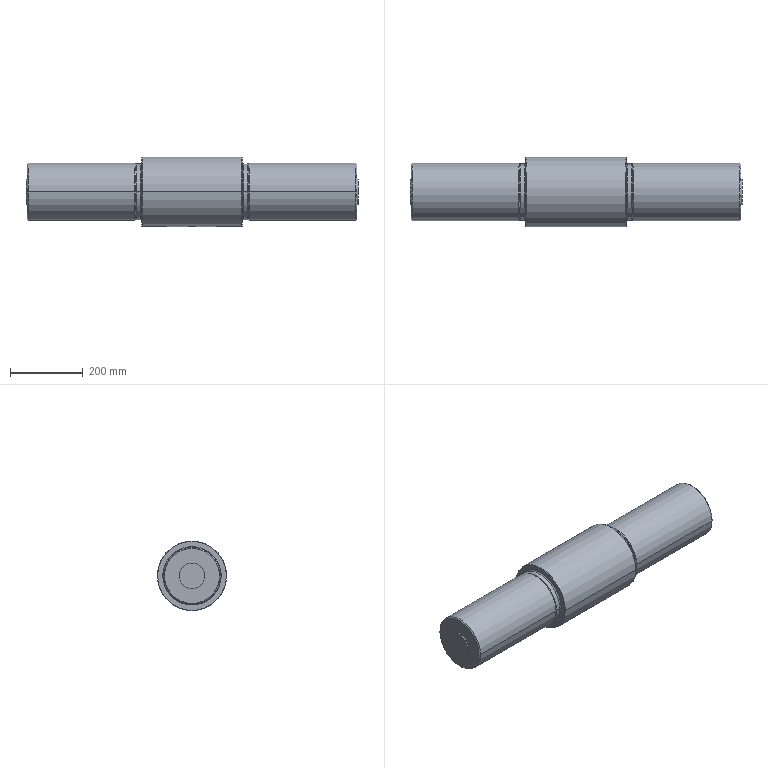Part | SolidWorks | features Chamfer 2, Cut 1, Fillet 1, Revolution 1 | 1 solid | 43 faces | box 909.904 x 190.424 x 190.424 mm | volume 20016200 mm3 | cylinder 16 | cone 12 | torus 8 | plane 7 | commonest cylinder face diameters 69.85 x4 154 x4 157.264 x4 22.631 x2 190.424 x2
STEP:
#1=CARTESIAN_POINT('',(0.,-11.316,-66.51));
#2=VERTEX_POINT('',#1);
#3=CARTESIAN_POINT('',(0.,11.316,-66.51));
#4=VERTEX_POINT('',#3);
#5=CARTESIAN_POINT('',(0.,0.,-66.51));
#6=DIRECTION('',(0.,0.,-1.));
#7=DIRECTION('',(0.,1.,0.));
#8=AXIS2_PLACEMENT_3D('',#5,#6,#7);
#9=CIRCLE('',#8,11.316);
#10=EDGE_CURVE('',#2,#4,#9,.T.);
#11=ORIENTED_EDGE('',*,*,#10,.F.);
#12=CARTESIAN_POINT('',(0.,-11.316,-94.537));
#13=VERTEX_POINT('',#12);
#14=CARTESIAN_POINT('',(0.,-11.316,-66.51));
#15=DIRECTION('',(0.,0.,-1.));
#16=VECTOR('',#15,1000.);
#17=LINE('',#14,#16);
#18=EDGE_CURVE('',#2,#13,#17,.T.);
#19=ORIENTED_EDGE('',*,*,#18,.T.);
#20=CARTESIAN_POINT('',(0.,11.316,-94.537));
#21=VERTEX_POINT('',#20);
#22=CARTESIAN_POINT('',(0.,11.316,-94.537));
#23=CARTESIAN_POINT('',(-0.7484,11.316,-94.537));
#24=CARTESIAN_POINT('',(-1.484,11.242,-94.546));
#25=CARTESIAN_POINT('',(-2.57,11.026,-94.571));
#26=CARTESIAN_POINT('',(-2.928,10.937,-94.582));
#27=CARTESIAN_POINT('',(-3.64,10.721,-94.606));
#28=CARTESIAN_POINT('',(-3.993,10.594,-94.621));
#29=CARTESIAN_POINT('',(-5.021,10.168,-94.668));
#30=CARTESIAN_POINT('',(-5.67,9.82,-94.705));
#31=CARTESIAN_POINT('',(-6.593,9.204,-94.766));
#32=CARTESIAN_POINT('',(-6.892,8.982,-94.788));
#33=CARTESIAN_POINT('',(-7.468,8.509,-94.831));
#34=CARTESIAN_POINT('',(-7.742,8.261,-94.853));
#35=CARTESIAN_POINT('',(-8.524,7.478,-94.919));
#36=CARTESIAN_POINT('',(-8.993,6.909,-94.963));
#37=CARTESIAN_POINT('',(-9.613,5.981,-95.024));
#38=CARTESIAN_POINT('',(-9.805,5.66,-95.044));
#39=CARTESIAN_POINT('',(-10.154,5.007,-95.081));
#40=CARTESIAN_POINT('',(-10.47,4.34,-95.115));
#41=CARTESIAN_POINT('',(-10.719,3.646,-95.143));
#42=CARTESIAN_POINT('',(-10.934,2.937,-95.167));
#43=CARTESIAN_POINT('',(-11.025,2.573,-95.178));
#44=CARTESIAN_POINT('',(-11.244,1.478,-95.203));
#45=CARTESIAN_POINT('',(-11.315,0.7429,-95.212));
#46=CARTESIAN_POINT('',(-11.316,-0.3652,-95.212));
#47=CARTESIAN_POINT('',(-11.298,-0.7357,-95.21));
#48=CARTESIAN_POINT('',(-11.225,-1.479,-95.201));
#49=CARTESIAN_POINT('',(-11.17,-1.848,-95.195));
#50=CARTESIAN_POINT('',(-10.953,-2.937,-95.169));
#51=CARTESIAN_POINT('',(-10.739,-3.643,-95.145));
#52=CARTESIAN_POINT('',(-10.313,-4.671,-95.098));
#53=CARTESIAN_POINT('',(-10.153,-5.01,-95.081));
#54=CARTESIAN_POINT('',(-9.803,-5.665,-95.044));
#55=CARTESIAN_POINT('',(-9.613,-5.982,-95.024));
#56=CARTESIAN_POINT('',(-8.998,-6.901,-94.963));
#57=CARTESIAN_POINT('',(-8.53,-7.472,-94.92));
#58=CARTESIAN_POINT('',(-7.474,-8.529,-94.831));
#59=CARTESIAN_POINT('',(-6.903,-8.996,-94.787));
#60=CARTESIAN_POINT('',(-5.985,-9.611,-94.726));
#61=CARTESIAN_POINT('',(-5.668,-9.801,-94.706));
#62=CARTESIAN_POINT('',(-5.013,-10.151,-94.669));
#63=CARTESIAN_POINT('',(-4.674,-10.312,-94.652));
#64=CARTESIAN_POINT('',(-3.646,-10.738,-94.605));
#65=CARTESIAN_POINT('',(-2.941,-10.952,-94.58));
#66=CARTESIAN_POINT('',(-1.852,-11.169,-94.555));
#67=CARTESIAN_POINT('',(-1.483,-11.224,-94.548));
#68=CARTESIAN_POINT('',(-0.7399,-11.298,-94.539));
#69=CARTESIAN_POINT('',(-0.3694,-11.316,-94.537));
#70=CARTESIAN_POINT('',(0.,-11.316,-94.537));
#71=B_SPLINE_CURVE_WITH_KNOTS('',3,(#22,#23,#24,#25,#26,#27,#28,#29,#30,#31,#32,#33,#34,#35,#36,#37,#38,#39,#40,#41,#42,#43,#44,#45,#46,#47,#48,#49,#50,#51,#52,#53,#54,#55,#56,#57,#58,#59,#60,#61,#62,#63,#64,#65,#66,#67,#68,#69,#70),.UNSPECIFIED.,.F.,.F.,(4,2,2,2,2,2,2,2,2,1,2,2,2,2,2,2,2,2,2,2,2,2,2,2,4),(0.,0.002213,0.00332,0.004426,0.006639,0.007746,0.008852,0.01107,0.01217,0.01328,0.01439,0.01549,0.0177,0.01881,0.01992,0.02213,0.02324,0.02434,0.02656,0.02877,0.02988,0.03098,0.0332,0.0343,0.03541),.UNSPECIFIED.);
#72=EDGE_CURVE('',#21,#13,#71,.T.);
#73=ORIENTED_EDGE('',*,*,#72,.F.);
#74=CARTESIAN_POINT('',(0.,11.316,-66.51));
#75=DIRECTION('',(0.,0.,-1.));
#76=VECTOR('',#75,1000.);
#77=LINE('',#74,#76);
#78=EDGE_CURVE('',#4,#21,#77,.T.);
#79=ORIENTED_EDGE('',*,*,#78,.F.);
#80=EDGE_LOOP('',(#11,#19,#73,#79));
#81=FACE_OUTER_BOUND('',#80,.T.);
#82=CARTESIAN_POINT('',(0.,0.,-66.51));
#83=DIRECTION('',(0.,0.,-1.));
#84=DIRECTION('',(0.,1.,0.));
#85=AXIS2_PLACEMENT_3D('',#82,#83,#84);
#86=CYLINDRICAL_SURFACE('',#85,11.316);
#87=ADVANCED_FACE('',(#81),#86,.F.);
#88=CARTESIAN_POINT('',(-137.325,-80.175,0.));
#89=VERTEX_POINT('',#88);
#90=CARTESIAN_POINT('',(-137.325,80.175,0.));
#91=VERTEX_POINT('',#90);
#92=CARTESIAN_POINT('',(-137.325,0.,0.));
#93=DIRECTION('',(1.,0.,0.));
#94=DIRECTION('',(0.,1.,0.));
#95=AXIS2_PLACEMENT_3D('',#92,#93,#94);
#96=CIRCLE('',#95,80.175);
#97=EDGE_CURVE('',#89,#91,#96,.T.);
#98=ORIENTED_EDGE('',*,*,#97,.F.);
#99=CARTESIAN_POINT('',(-140.5,-77.,0.));
#100=VERTEX_POINT('',#99);
#101=CARTESIAN_POINT('',(-140.5,-80.175,0.));
#102=DIRECTION('',(0.,0.,1.));
#103=DIRECTION('',(0.,-1.,0.));
#104=AXIS2_PLACEMENT_3D('',#101,#102,#103);
#105=CIRCLE('',#104,3.175);
#106=EDGE_CURVE('',#89,#100,#105,.T.);
#107=ORIENTED_EDGE('',*,*,#106,.T.);
#108=CARTESIAN_POINT('',(-140.5,77.,0.));
#109=VERTEX_POINT('',#108);
#110=CARTESIAN_POINT('',(-140.5,0.,0.));
#111=DIRECTION('',(-1.,0.,0.));
#112=DIRECTION('',(0.,1.,0.));
#113=AXIS2_PLACEMENT_3D('',#110,#111,#112);
#114=CIRCLE('',#113,77.);
#115=EDGE_CURVE('',#109,#100,#114,.T.);
#116=ORIENTED_EDGE('',*,*,#115,.F.);
#117=CARTESIAN_POINT('',(-140.5,80.175,0.));
#118=DIRECTION('',(0.,0.,-1.));
#119=DIRECTION('',(-1.,0.,0.));
#120=AXIS2_PLACEMENT_3D('',#117,#118,#119);
#121=CIRCLE('',#120,3.175);
#122=EDGE_CURVE('',#91,#109,#121,.T.);
#123=ORIENTED_EDGE('',*,*,#122,.F.);
#124=EDGE_LOOP('',(#98,#107,#116,#123));
#125=FACE_OUTER_BOUND('',#124,.T.);
#126=CARTESIAN_POINT('',(-140.5,0.,0.));
#127=DIRECTION('',(1.,0.,0.));
#128=DIRECTION('',(0.,1.,0.));
#129=AXIS2_PLACEMENT_3D('',#126,#127,#128);
#130=TOROIDAL_SURFACE('',#129,80.175,3.175);
#131=ADVANCED_FACE('',(#125),#130,.F.);
#132=CARTESIAN_POINT('',(-154.285,77.425,0.));
#133=VERTEX_POINT('',#132);
#134=CARTESIAN_POINT('',(-154.285,-77.425,0.));
#135=VERTEX_POINT('',#134);
#136=CARTESIAN_POINT('',(-154.285,0.,0.));
#137=DIRECTION('',(-1.,0.,0.));
#138=DIRECTION('',(0.,-1.,0.));
#139=AXIS2_PLACEMENT_3D('',#136,#137,#138);
#140=CIRCLE('',#139,77.425);
#141=EDGE_CURVE('',#133,#135,#140,.T.);
#142=ORIENTED_EDGE('',*,*,#141,.F.);
#143=CARTESIAN_POINT('',(-152.698,77.,0.));
#144=VERTEX_POINT('',#143);
#145=CARTESIAN_POINT('',(-152.698,80.175,0.));
#146=DIRECTION('',(0.,0.,1.));
#147=DIRECTION('',(0.,-1.,0.));
#148=AXIS2_PLACEMENT_3D('',#145,#146,#147);
#149=CIRCLE('',#148,3.175);
#150=EDGE_CURVE('',#133,#144,#149,.T.);
#151=ORIENTED_EDGE('',*,*,#150,.T.);
#152=CARTESIAN_POINT('',(-152.698,-77.,0.));
#153=VERTEX_POINT('',#152);
#154=CARTESIAN_POINT('',(-152.698,0.,0.));
#155=DIRECTION('',(1.,0.,0.));
#156=DIRECTION('',(0.,-1.,0.));
#157=AXIS2_PLACEMENT_3D('',#154,#155,#156);
#158=CIRCLE('',#157,77.);
#159=EDGE_CURVE('',#153,#144,#158,.T.);
#160=ORIENTED_EDGE('',*,*,#159,.F.);
#161=CARTESIAN_POINT('',(-152.698,-80.175,0.));
#162=DIRECTION('',(0.,0.,-1.));
#163=DIRECTION('',(-1.,0.,0.));
#164=AXIS2_PLACEMENT_3D('',#161,#162,#163);
#165=CIRCLE('',#164,3.175);
#166=EDGE_CURVE('',#135,#153,#165,.T.);
#167=ORIENTED_EDGE('',*,*,#166,.F.);
#168=EDGE_LOOP('',(#142,#151,#160,#167));
#169=FACE_OUTER_BOUND('',#168,.T.);
#170=CARTESIAN_POINT('',(-152.698,0.,0.));
#171=DIRECTION('',(-1.,0.,0.));
#172=DIRECTION('',(0.,-1.,0.));
#173=AXIS2_PLACEMENT_3D('',#170,#171,#172);
#174=TOROIDAL_SURFACE('',#173,80.175,3.175);
#175=ADVANCED_FACE('',(#169),#174,.F.);
#176=CARTESIAN_POINT('',(137.325,80.175,0.));
#177=VERTEX_POINT('',#176);
#178=CARTESIAN_POINT('',(137.325,-80.175,0.));
#179=VERTEX_POINT('',#178);
#180=CARTESIAN_POINT('',(137.325,0.,0.));
#181=DIRECTION('',(-1.,0.,0.));
#182=DIRECTION('',(0.,-1.,0.));
#183=AXIS2_PLACEMENT_3D('',#180,#181,#182);
#184=CIRCLE('',#183,80.175);
#185=EDGE_CURVE('',#177,#179,#184,.T.);
#186=ORIENTED_EDGE('',*,*,#185,.F.);
#187=CARTESIAN_POINT('',(140.5,77.,0.));
#188=VERTEX_POINT('',#187);
#189=CARTESIAN_POINT('',(140.5,80.175,0.));
#190=DIRECTION('',(0.,0.,1.));
#191=DIRECTION('',(0.,-1.,0.));
#192=AXIS2_PLACEMENT_3D('',#189,#190,#191);
#193=CIRCLE('',#192,3.175);
#194=EDGE_CURVE('',#177,#188,#193,.T.);
#195=ORIENTED_EDGE('',*,*,#194,.T.);
#196=CARTESIAN_POINT('',(140.5,-77.,0.));
#197=VERTEX_POINT('',#196);
#198=CARTESIAN_POINT('',(140.5,0.,0.));
#199=DIRECTION('',(1.,0.,0.));
#200=DIRECTION('',(0.,-1.,0.));
#201=AXIS2_PLACEMENT_3D('',#198,#199,#200);
#202=CIRCLE('',#201,77.);
#203=EDGE_CURVE('',#197,#188,#202,.T.);
#204=ORIENTED_EDGE('',*,*,#203,.F.);
#205=CARTESIAN_POINT('',(140.5,-80.175,0.));
#206=DIRECTION('',(0.,0.,-1.));
#207=DIRECTION('',(-1.,0.,0.));
#208=AXIS2_PLACEMENT_3D('',#205,#206,#207);
#209=CIRCLE('',#208,3.175);
#210=EDGE_CURVE('',#179,#197,#209,.T.);
#211=ORIENTED_EDGE('',*,*,#210,.F.);
#212=EDGE_LOOP('',(#186,#195,#204,#211));
#213=FACE_OUTER_BOUND('',#212,.T.);
#214=CARTESIAN_POINT('',(140.5,0.,0.));
#215=DIRECTION('',(-1.,0.,0.));
#216=DIRECTION('',(0.,-1.,0.));
#217=AXIS2_PLACEMENT_3D('',#214,#215,#216);
#218=TOROIDAL_SURFACE('',#217,80.175,3.175);
#219=ADVANCED_FACE('',(#213),#218,.F.);
#220=CARTESIAN_POINT('',(152.698,77.,0.));
#221=VERTEX_POINT('',#220);
#222=CARTESIAN_POINT('',(152.698,-77.,0.));
#223=VERTEX_POINT('',#222);
#224=CARTESIAN_POINT('',(152.698,0.,0.));
#225=DIRECTION('',(-1.,0.,0.));
#226=DIRECTION('',(0.,-1.,0.));
#227=AXIS2_PLACEMENT_3D('',#224,#225,#226);
#228=CIRCLE('',#227,77.);
#229=EDGE_CURVE('',#221,#223,#228,.T.);
#230=ORIENTED_EDGE('',*,*,#229,.F.);
#231=CARTESIAN_POINT('',(154.285,77.425,0.));
#232=VERTEX_POINT('',#231);
#233=CARTESIAN_POINT('',(152.698,80.175,0.));
#234=DIRECTION('',(0.,0.,1.));
#235=DIRECTION('',(0.,-1.,0.));
#236=AXIS2_PLACEMENT_3D('',#233,#234,#235);
#237=CIRCLE('',#236,3.175);
#238=EDGE_CURVE('',#221,#232,#237,.T.);
#239=ORIENTED_EDGE('',*,*,#238,.T.);
#240=CARTESIAN_POINT('',(154.285,-77.425,0.));
#241=VERTEX_POINT('',#240);
#242=CARTESIAN_POINT('',(154.285,0.,0.));
#243=DIRECTION('',(1.,0.,0.));
#244=DIRECTION('',(0.,1.,0.));
#245=AXIS2_PLACEMENT_3D('',#242,#243,#244);
#246=CIRCLE('',#245,77.425);
#247=EDGE_CURVE('',#241,#232,#246,.T.);
#248=ORIENTED_EDGE('',*,*,#247,.F.);
#249=CARTESIAN_POINT('',(152.698,-80.175,0.));
#250=DIRECTION('',(0.,0.,-1.));
#251=DIRECTION('',(-1.,0.,0.));
#252=AXIS2_PLACEMENT_3D('',#249,#250,#251);
#253=CIRCLE('',#252,3.175);
#254=EDGE_CURVE('',#223,#241,#253,.T.);
#255=ORIENTED_EDGE('',*,*,#254,.F.);
#256=EDGE_LOOP('',(#230,#239,#248,#255));
#257=FACE_OUTER_BOUND('',#256,.T.);
#258=CARTESIAN_POINT('',(152.698,0.,0.));
#259=DIRECTION('',(-1.,0.,0.));
#260=DIRECTION('',(0.,-1.,0.));
#261=AXIS2_PLACEMENT_3D('',#258,#259,#260);
#262=TOROIDAL_SURFACE('',#261,80.175,3.175);
#263=ADVANCED_FACE('',(#257),#262,.F.);
#264=CARTESIAN_POINT('',(-137.325,-94.45,0.));
#265=VERTEX_POINT('',#264);
#266=CARTESIAN_POINT('',(-137.325,94.45,0.));
#267=VERTEX_POINT('',#266);
#268=CARTESIAN_POINT('',(-137.325,0.,0.));
#269=DIRECTION('',(-1.,0.,0.));
#270=DIRECTION('',(0.,1.,0.));
#271=AXIS2_PLACEMENT_3D('',#268,#269,#270);
#272=CIRCLE('',#271,94.45);
#273=EDGE_CURVE('',#265,#267,#272,.T.);
#274=ORIENTED_EDGE('',*,*,#273,.F.);
#275=CARTESIAN_POINT('',(-136.563,-95.212,0.));
#276=VERTEX_POINT('',#275);
#277=CARTESIAN_POINT('',(-137.325,-94.45,0.));
#278=DIRECTION('',(0.7071,-0.7071,0.));
#279=VECTOR('',#278,1000.);
#280=LINE('',#277,#279);
#281=EDGE_CURVE('',#265,#276,#280,.T.);
#282=ORIENTED_EDGE('',*,*,#281,.T.);
#283=CARTESIAN_POINT('',(-136.563,95.212,0.));
#284=VERTEX_POINT('',#283);
#285=CARTESIAN_POINT('',(-136.563,0.,0.));
#286=DIRECTION('',(1.,0.,0.));
#287=DIRECTION('',(0.,1.,0.));
#288=AXIS2_PLACEMENT_3D('',#285,#286,#287);
#289=CIRCLE('',#288,95.212);
#290=EDGE_CURVE('',#284,#276,#289,.T.);
#291=ORIENTED_EDGE('',*,*,#290,.F.);
#292=CARTESIAN_POINT('',(-137.325,94.45,0.));
#293=DIRECTION('',(0.7071,0.7071,0.));
#294=VECTOR('',#293,1000.);
#295=LINE('',#292,#294);
#296=EDGE_CURVE('',#267,#284,#295,.T.);
#297=ORIENTED_EDGE('',*,*,#296,.F.);
#298=EDGE_LOOP('',(#274,#282,#291,#297));
#299=FACE_OUTER_BOUND('',#298,.T.);
#300=CARTESIAN_POINT('',(-137.325,0.,0.));
#301=DIRECTION('',(1.,0.,0.));
#302=DIRECTION('',(0.,1.,0.));
#303=AXIS2_PLACEMENT_3D('',#300,#301,#302);
#304=CONICAL_SURFACE('',#303,94.45,0.7854);
#305=ADVANCED_FACE('',(#299),#304,.T.);
#306=CARTESIAN_POINT('',(137.325,94.45,0.));
#307=VERTEX_POINT('',#306);
#308=CARTESIAN_POINT('',(137.325,-94.45,0.));
#309=VERTEX_POINT('',#308);
#310=CARTESIAN_POINT('',(137.325,0.,0.));
#311=DIRECTION('',(1.,0.,0.));
#312=DIRECTION('',(0.,-1.,0.));
#313=AXIS2_PLACEMENT_3D('',#310,#311,#312);
#314=CIRCLE('',#313,94.45);
#315=EDGE_CURVE('',#307,#309,#314,.T.);
#316=ORIENTED_EDGE('',*,*,#315,.F.);
#317=CARTESIAN_POINT('',(136.563,95.212,0.));
#318=VERTEX_POINT('',#317);
#319=CARTESIAN_POINT('',(136.563,95.212,0.));
#320=DIRECTION('',(-0.7071,0.7071,0.));
#321=VECTOR('',#320,1000.);
#322=LINE('',#319,#321);
#323=EDGE_CURVE('',#307,#318,#322,.T.);
#324=ORIENTED_EDGE('',*,*,#323,.T.);
#325=CARTESIAN_POINT('',(136.563,-95.212,0.));
#326=VERTEX_POINT('',#325);
#327=CARTESIAN_POINT('',(136.563,0.,0.));
#328=DIRECTION('',(-1.,0.,0.));
#329=DIRECTION('',(0.,-1.,0.));
#330=AXIS2_PLACEMENT_3D('',#327,#328,#329);
#331=CIRCLE('',#330,95.212);
#332=EDGE_CURVE('',#326,#318,#331,.T.);
#333=ORIENTED_EDGE('',*,*,#332,.F.);
#334=CARTESIAN_POINT('',(136.563,-95.212,0.));
#335=DIRECTION('',(-0.7071,-0.7071,0.));
#336=VECTOR('',#335,1000.);
#337=LINE('',#334,#336);
#338=EDGE_CURVE('',#309,#326,#337,.T.);
#339=ORIENTED_EDGE('',*,*,#338,.F.);
#340=EDGE_LOOP('',(#316,#324,#333,#339));
#341=FACE_OUTER_BOUND('',#340,.T.);
#342=CARTESIAN_POINT('',(136.563,0.,0.));
#343=DIRECTION('',(-1.,0.,0.));
#344=DIRECTION('',(0.,-1.,0.));
#345=AXIS2_PLACEMENT_3D('',#342,#343,#344);
#346=CONICAL_SURFACE('',#345,95.212,0.7854);
#347=ADVANCED_FACE('',(#341),#346,.T.);
#348=CARTESIAN_POINT('',(-451.65,-75.632,0.));
#349=VERTEX_POINT('',#348);
#350=CARTESIAN_POINT('',(-451.65,75.632,0.));
#351=VERTEX_POINT('',#350);
#352=CARTESIAN_POINT('',(-451.65,0.,0.));
#353=DIRECTION('',(-1.,0.,0.));
#354=DIRECTION('',(0.,1.,0.));
#355=AXIS2_PLACEMENT_3D('',#352,#353,#354);
#356=CIRCLE('',#355,75.632);
#357=EDGE_CURVE('',#349,#351,#356,.T.);
#358=ORIENTED_EDGE('',*,*,#357,.F.);
#359=CARTESIAN_POINT('',(-448.65,-78.632,0.));
#360=VERTEX_POINT('',#359);
#361=CARTESIAN_POINT('',(-451.65,-75.632,0.));
#362=DIRECTION('',(0.7071,-0.7071,0.));
#363=VECTOR('',#362,1000.);
#364=LINE('',#361,#363);
#365=EDGE_CURVE('',#349,#360,#364,.T.);
#366=ORIENTED_EDGE('',*,*,#365,.T.);
#367=CARTESIAN_POINT('',(-448.65,78.632,0.));
#368=VERTEX_POINT('',#367);
#369=CARTESIAN_POINT('',(-448.65,0.,0.));
#370=DIRECTION('',(1.,0.,0.));
#371=DIRECTION('',(0.,1.,0.));
#372=AXIS2_PLACEMENT_3D('',#369,#370,#371);
#373=CIRCLE('',#372,78.632);
#374=EDGE_CURVE('',#368,#360,#373,.T.);
#375=ORIENTED_EDGE('',*,*,#374,.F.);
#376=CARTESIAN_POINT('',(-451.65,75.632,0.));
#377=DIRECTION('',(0.7071,0.7071,0.));
#378=VECTOR('',#377,1000.);
#379=LINE('',#376,#378);
#380=EDGE_CURVE('',#351,#368,#379,.T.);
#381=ORIENTED_EDGE('',*,*,#380,.F.);
#382=EDGE_LOOP('',(#358,#366,#375,#381));
#383=FACE_OUTER_BOUND('',#382,.T.);
#384=CARTESIAN_POINT('',(-451.65,0.,0.));
#385=DIRECTION('',(1.,0.,0.));
#386=DIRECTION('',(0.,1.,0.));
#387=AXIS2_PLACEMENT_3D('',#384,#385,#386);
#388=CONICAL_SURFACE('',#387,75.632,0.7854);
#389=ADVANCED_FACE('',(#383),#388,.T.);
#390=CARTESIAN_POINT('',(451.65,75.632,0.));
#391=VERTEX_POINT('',#390);
#392=CARTESIAN_POINT('',(451.65,-75.632,0.));
#393=VERTEX_POINT('',#392);
#394=CARTESIAN_POINT('',(451.65,0.,0.));
#395=DIRECTION('',(1.,0.,0.));
#396=DIRECTION('',(0.,-1.,0.));
#397=AXIS2_PLACEMENT_3D('',#394,#395,#396);
#398=CIRCLE('',#397,75.632);
#399=EDGE_CURVE('',#391,#393,#398,.T.);
#400=ORIENTED_EDGE('',*,*,#399,.F.);
#401=CARTESIAN_POINT('',(448.65,78.632,0.));
#402=VERTEX_POINT('',#401);
#403=CARTESIAN_POINT('',(448.65,78.632,0.));
#404=DIRECTION('',(-0.7071,0.7071,0.));
#405=VECTOR('',#404,1000.);
#406=LINE('',#403,#405);
#407=EDGE_CURVE('',#391,#402,#406,.T.);
#408=ORIENTED_EDGE('',*,*,#407,.T.);
#409=CARTESIAN_POINT('',(448.65,-78.632,0.));
#410=VERTEX_POINT('',#409);
#411=CARTESIAN_POINT('',(448.65,0.,0.));
#412=DIRECTION('',(-1.,0.,0.));
#413=DIRECTION('',(0.,-1.,0.));
#414=AXIS2_PLACEMENT_3D('',#411,#412,#413);
#415=CIRCLE('',#414,78.632);
#416=EDGE_CURVE('',#410,#402,#415,.T.);
#417=ORIENTED_EDGE('',*,*,#416,.F.);
#418=CARTESIAN_POINT('',(448.65,-78.632,0.));
#419=DIRECTION('',(-0.7071,-0.7071,0.));
#420=VECTOR('',#419,1000.);
#421=LINE('',#418,#420);
#422=EDGE_CURVE('',#393,#410,#421,.T.);
#423=ORIENTED_EDGE('',*,*,#422,.F.);
#424=EDGE_LOOP('',(#400,#408,#417,#423));
#425=FACE_OUTER_BOUND('',#424,.T.);
#426=CARTESIAN_POINT('',(448.65,0.,0.));
#427=DIRECTION('',(-1.,0.,0.));
#428=DIRECTION('',(0.,-1.,0.));
#429=AXIS2_PLACEMENT_3D('',#426,#427,#428);
#430=CONICAL_SURFACE('',#429,78.632,0.7854);
#431=ADVANCED_FACE('',(#425),#430,.T.);
#432=CARTESIAN_POINT('',(154.285,0.,0.));
#433=DIRECTION('',(1.,0.,0.));
#434=DIRECTION('',(0.,1.,0.));
#435=AXIS2_PLACEMENT_3D('',#432,#433,#434);
#436=CIRCLE('',#435,77.425);
#437=EDGE_CURVE('',#232,#241,#436,.T.);
#438=ORIENTED_EDGE('',*,*,#437,.T.);
#439=CARTESIAN_POINT('',(156.375,-78.632,0.));
#440=VERTEX_POINT('',#439);
#441=CARTESIAN_POINT('',(156.375,-78.632,0.));
#442=DIRECTION('',(0.866,-0.5,0.));
#443=VECTOR('',#442,1000.);
#444=LINE('',#441,#443);
#445=EDGE_CURVE('',#241,#440,#444,.T.);
#446=ORIENTED_EDGE('',*,*,#445,.T.);
#447=CARTESIAN_POINT('',(156.375,78.632,0.));
#448=VERTEX_POINT('',#447);
#449=CARTESIAN_POINT('',(156.375,0.,0.));
#450=DIRECTION('',(-1.,0.,0.));
#451=DIRECTION('',(0.,-1.,0.));
#452=AXIS2_PLACEMENT_3D('',#449,#450,#451);
#453=CIRCLE('',#452,78.632);
#454=EDGE_CURVE('',#440,#448,#453,.T.);
#455=ORIENTED_EDGE('',*,*,#454,.T.);
#456=CARTESIAN_POINT('',(156.375,78.632,0.));
#457=DIRECTION('',(0.866,0.5,0.));
#458=VECTOR('',#457,1000.);
#459=LINE('',#456,#458);
#460=EDGE_CURVE('',#232,#448,#459,.T.);
#461=ORIENTED_EDGE('',*,*,#460,.F.);
#462=EDGE_LOOP('',(#438,#446,#455,#461));
#463=FACE_OUTER_BOUND('',#462,.T.);
#464=CARTESIAN_POINT('',(156.375,0.,0.));
#465=DIRECTION('',(1.,0.,0.));
#466=DIRECTION('',(0.,1.,0.));
#467=AXIS2_PLACEMENT_3D('',#464,#465,#466);
#468=CONICAL_SURFACE('',#467,78.632,0.5236);
#469=ADVANCED_FACE('',(#463),#468,.T.);
#470=CARTESIAN_POINT('',(152.698,0.,0.));
#471=DIRECTION('',(-1.,0.,0.));
#472=DIRECTION('',(0.,-1.,0.));
#473=AXIS2_PLACEMENT_3D('',#470,#471,#472);
#474=CIRCLE('',#473,77.);
#475=EDGE_CURVE('',#223,#221,#474,.T.);
#476=ORIENTED_EDGE('',*,*,#475,.T.);
#477=CARTESIAN_POINT('',(-454.952,77.,0.));
#478=DIRECTION('',(-1.,0.,0.));
#479=VECTOR('',#478,1000.);
#480=LINE('',#477,#479);
#481=EDGE_CURVE('',#221,#188,#480,.T.);
#482=ORIENTED_EDGE('',*,*,#481,.T.);
#483=CARTESIAN_POINT('',(140.5,0.,0.));
#484=DIRECTION('',(1.,0.,0.));
#485=DIRECTION('',(0.,-1.,0.));
#486=AXIS2_PLACEMENT_3D('',#483,#484,#485);
#487=CIRCLE('',#486,77.);
#488=EDGE_CURVE('',#188,#197,#487,.T.);
#489=ORIENTED_EDGE('',*,*,#488,.T.);
#490=CARTESIAN_POINT('',(-454.952,-77.,0.));
#491=DIRECTION('',(-1.,0.,0.));
#492=VECTOR('',#491,1000.);
#493=LINE('',#490,#492);
#494=EDGE_CURVE('',#223,#197,#493,.T.);
#495=ORIENTED_EDGE('',*,*,#494,.F.);
#496=EDGE_LOOP('',(#476,#482,#489,#495));
#497=FACE_OUTER_BOUND('',#496,.T.);
#498=CARTESIAN_POINT('',(-454.952,0.,0.));
#499=DIRECTION('',(-1.,0.,0.));
#500=DIRECTION('',(0.,-1.,0.));
#501=AXIS2_PLACEMENT_3D('',#498,#499,#500);
#502=CYLINDRICAL_SURFACE('',#501,77.);
#503=ADVANCED_FACE('',(#497),#502,.T.);
#504=ORIENTED_EDGE('',*,*,#332,.T.);
#505=CARTESIAN_POINT('',(-454.952,95.212,0.));
#506=DIRECTION('',(-1.,0.,0.));
#507=VECTOR('',#506,1000.);
#508=LINE('',#505,#507);
#509=EDGE_CURVE('',#318,#284,#508,.T.);
#510=ORIENTED_EDGE('',*,*,#509,.T.);
#511=ORIENTED_EDGE('',*,*,#290,.T.);
#512=CARTESIAN_POINT('',(-454.952,-95.212,0.));
#513=DIRECTION('',(-1.,0.,0.));
#514=VECTOR('',#513,1000.);
#515=LINE('',#512,#514);
#516=EDGE_CURVE('',#326,#276,#515,.T.);
#517=ORIENTED_EDGE('',*,*,#516,.F.);
#518=EDGE_LOOP('',(#504,#510,#511,#517));
#519=FACE_OUTER_BOUND('',#518,.T.);
#520=CARTESIAN_POINT('',(-454.952,0.,0.));
#521=DIRECTION('',(-1.,0.,0.));
#522=DIRECTION('',(0.,-1.,0.));
#523=AXIS2_PLACEMENT_3D('',#520,#521,#522);
#524=CYLINDRICAL_SURFACE('',#523,95.212);
#525=ADVANCED_FACE('',(#519),#524,.T.);
#526=CARTESIAN_POINT('',(-140.5,0.,0.));
#527=DIRECTION('',(-1.,0.,0.));
#528=DIRECTION('',(0.,1.,0.));
#529=AXIS2_PLACEMENT_3D('',#526,#527,#528);
#530=CIRCLE('',#529,77.);
#531=EDGE_CURVE('',#100,#109,#530,.T.);
#532=ORIENTED_EDGE('',*,*,#531,.T.);
#533=CARTESIAN_POINT('',(-454.952,77.,0.));
#534=DIRECTION('',(-1.,0.,0.));
#535=VECTOR('',#534,1000.);
#536=LINE('',#533,#535);
#537=EDGE_CURVE('',#109,#144,#536,.T.);
#538=ORIENTED_EDGE('',*,*,#537,.T.);
#539=CARTESIAN_POINT('',(-152.698,0.,0.));
#540=DIRECTION('',(1.,0.,0.));
#541=DIRECTION('',(0.,-1.,0.));
#542=AXIS2_PLACEMENT_3D('',#539,#540,#541);
#543=CIRCLE('',#542,77.);
#544=EDGE_CURVE('',#144,#153,#543,.T.);
#545=ORIENTED_EDGE('',*,*,#544,.T.);
#546=CARTESIAN_POINT('',(-454.952,-77.,0.));
#547=DIRECTION('',(-1.,0.,0.));
#548=VECTOR('',#547,1000.);
#549=LINE('',#546,#548);
#550=EDGE_CURVE('',#100,#153,#549,.T.);
#551=ORIENTED_EDGE('',*,*,#550,.F.);
#552=EDGE_LOOP('',(#532,#538,#545,#551));
#553=FACE_OUTER_BOUND('',#552,.T.);
#554=CARTESIAN_POINT('',(-454.952,0.,0.));
#555=DIRECTION('',(-1.,0.,0.));
#556=DIRECTION('',(0.,-1.,0.));
#557=AXIS2_PLACEMENT_3D('',#554,#555,#556);
#558=CYLINDRICAL_SURFACE('',#557,77.);
#559=ADVANCED_FACE('',(#553),#558,.T.);
#560=CARTESIAN_POINT('',(-154.285,0.,0.));
#561=DIRECTION('',(-1.,0.,0.));
#562=DIRECTION('',(0.,-1.,0.));
#563=AXIS2_PLACEMENT_3D('',#560,#561,#562);
#564=CIRCLE('',#563,77.425);
#565=EDGE_CURVE('',#135,#133,#564,.T.);
#566=ORIENTED_EDGE('',*,*,#565,.T.);
#567=CARTESIAN_POINT('',(-156.375,78.632,0.));
#568=VERTEX_POINT('',#567);
#569=CARTESIAN_POINT('',(-153.548,77.,0.));
#570=DIRECTION('',(-0.866,0.5,0.));
#571=VECTOR('',#570,1000.);
#572=LINE('',#569,#571);
#573=EDGE_CURVE('',#133,#568,#572,.T.);
#574=ORIENTED_EDGE('',*,*,#573,.T.);
#575=CARTESIAN_POINT('',(-156.375,-78.632,0.));
#576=VERTEX_POINT('',#575);
#577=CARTESIAN_POINT('',(-156.375,0.,0.));
#578=DIRECTION('',(-1.,0.,0.));
#579=DIRECTION('',(0.,-1.,0.));
#580=AXIS2_PLACEMENT_3D('',#577,#578,#579);
#581=CIRCLE('',#580,78.632);
#582=EDGE_CURVE('',#576,#568,#581,.T.);
#583=ORIENTED_EDGE('',*,*,#582,.F.);
#584=CARTESIAN_POINT('',(-153.548,-77.,0.));
#585=DIRECTION('',(-0.866,-0.5,0.));
#586=VECTOR('',#585,1000.);
#587=LINE('',#584,#586);
#588=EDGE_CURVE('',#135,#576,#587,.T.);
#589=ORIENTED_EDGE('',*,*,#588,.F.);
#590=EDGE_LOOP('',(#566,#574,#583,#589));
#591=FACE_OUTER_BOUND('',#590,.T.);
#592=CARTESIAN_POINT('',(-153.548,0.,0.));
#593=DIRECTION('',(-1.,0.,0.));
#594=DIRECTION('',(0.,-1.,0.));
#595=AXIS2_PLACEMENT_3D('',#592,#593,#594);
#596=CONICAL_SURFACE('',#595,77.,0.5236);
#597=ADVANCED_FACE('',(#591),#596,.T.);
#598=ORIENTED_EDGE('',*,*,#582,.T.);
#599=CARTESIAN_POINT('',(-454.952,78.632,0.));
#600=DIRECTION('',(-1.,0.,0.));
#601=VECTOR('',#600,1000.);
#602=LINE('',#599,#601);
#603=EDGE_CURVE('',#568,#368,#602,.T.);
#604=ORIENTED_EDGE('',*,*,#603,.T.);
#605=ORIENTED_EDGE('',*,*,#374,.T.);
#606=CARTESIAN_POINT('',(-454.952,-78.632,0.));
#607=DIRECTION('',(-1.,0.,0.));
#608=VECTOR('',#607,1000.);
#609=LINE('',#606,#608);
#610=EDGE_CURVE('',#576,#360,#609,.T.);
#611=ORIENTED_EDGE('',*,*,#610,.F.);
#612=EDGE_LOOP('',(#598,#604,#605,#611));
#613=FACE_OUTER_BOUND('',#612,.T.);
#614=CARTESIAN_POINT('',(-454.952,0.,0.));
#615=DIRECTION('',(-1.,0.,0.));
#616=DIRECTION('',(0.,-1.,0.));
#617=AXIS2_PLACEMENT_3D('',#614,#615,#616);
#618=CYLINDRICAL_SURFACE('',#617,78.632);
#619=ADVANCED_FACE('',(#613),#618,.T.);
#620=CARTESIAN_POINT('',(-451.65,-34.925,0.));
#621=VERTEX_POINT('',#620);
#622=CARTESIAN_POINT('',(-451.65,34.925,0.));
#623=VERTEX_POINT('',#622);
#624=CARTESIAN_POINT('',(-451.65,0.,0.));
#625=DIRECTION('',(-1.,0.,0.));
#626=DIRECTION('',(0.,-1.,0.));
#627=AXIS2_PLACEMENT_3D('',#624,#625,#626);
#628=CIRCLE('',#627,34.925);
#629=EDGE_CURVE('',#621,#623,#628,.T.);
#630=ORIENTED_EDGE('',*,*,#629,.T.);
#631=CARTESIAN_POINT('',(-454.952,34.925,0.));
#632=VERTEX_POINT('',#631);
#633=CARTESIAN_POINT('',(-454.952,34.925,0.));
#634=DIRECTION('',(-1.,0.,0.));
#635=VECTOR('',#634,1000.);
#636=LINE('',#633,#635);
#637=EDGE_CURVE('',#623,#632,#636,.T.);
#638=ORIENTED_EDGE('',*,*,#637,.T.);
#639=CARTESIAN_POINT('',(-454.952,-34.925,0.));
#640=VERTEX_POINT('',#639);
#641=CARTESIAN_POINT('',(-454.952,0.,0.));
#642=DIRECTION('',(-1.,0.,0.));
#643=DIRECTION('',(0.,-1.,0.));
#644=AXIS2_PLACEMENT_3D('',#641,#642,#643);
#645=CIRCLE('',#644,34.925);
#646=EDGE_CURVE('',#640,#632,#645,.T.);
#647=ORIENTED_EDGE('',*,*,#646,.F.);
#648=CARTESIAN_POINT('',(-454.952,-34.925,0.));
#649=DIRECTION('',(-1.,0.,0.));
#650=VECTOR('',#649,1000.);
#651=LINE('',#648,#650);
#652=EDGE_CURVE('',#621,#640,#651,.T.);
#653=ORIENTED_EDGE('',*,*,#652,.F.);
#654=EDGE_LOOP('',(#630,#638,#647,#653));
#655=FACE_OUTER_BOUND('',#654,.T.);
#656=CARTESIAN_POINT('',(-454.952,0.,0.));
#657=DIRECTION('',(-1.,0.,0.));
#658=DIRECTION('',(0.,-1.,0.));
#659=AXIS2_PLACEMENT_3D('',#656,#657,#658);
#660=CYLINDRICAL_SURFACE('',#659,34.925);
#661=ADVANCED_FACE('',(#655),#660,.T.);
#662=CARTESIAN_POINT('',(454.952,-34.925,0.));
#663=VERTEX_POINT('',#662);
#664=CARTESIAN_POINT('',(454.952,34.925,0.));
#665=VERTEX_POINT('',#664);
#666=CARTESIAN_POINT('',(454.952,0.,0.));
#667=DIRECTION('',(-1.,0.,0.));
#668=DIRECTION('',(0.,-1.,0.));
#669=AXIS2_PLACEMENT_3D('',#666,#667,#668);
#670=CIRCLE('',#669,34.925);
#671=EDGE_CURVE('',#663,#665,#670,.T.);
#672=ORIENTED_EDGE('',*,*,#671,.T.);
#673=CARTESIAN_POINT('',(451.65,34.925,0.));
#674=VERTEX_POINT('',#673);
#675=CARTESIAN_POINT('',(-454.952,34.925,0.));
#676=DIRECTION('',(-1.,0.,0.));
#677=VECTOR('',#676,1000.);
#678=LINE('',#675,#677);
#679=EDGE_CURVE('',#665,#674,#678,.T.);
#680=ORIENTED_EDGE('',*,*,#679,.T.);
#681=CARTESIAN_POINT('',(451.65,-34.925,0.));
#682=VERTEX_POINT('',#681);
#683=CARTESIAN_POINT('',(451.65,0.,0.));
#684=DIRECTION('',(-1.,0.,0.));
#685=DIRECTION('',(0.,-1.,0.));
#686=AXIS2_PLACEMENT_3D('',#683,#684,#685);
#687=CIRCLE('',#686,34.925);
#688=EDGE_CURVE('',#682,#674,#687,.T.);
#689=ORIENTED_EDGE('',*,*,#688,.F.);
#690=CARTESIAN_POINT('',(-454.952,-34.925,0.));
#691=DIRECTION('',(-1.,0.,0.));
#692=VECTOR('',#691,1000.);
#693=LINE('',#690,#692);
#694=EDGE_CURVE('',#663,#682,#693,.T.);
#695=ORIENTED_EDGE('',*,*,#694,.F.);
#696=EDGE_LOOP('',(#672,#680,#689,#695));
#697=FACE_OUTER_BOUND('',#696,.T.);
#698=CARTESIAN_POINT('',(-454.952,0.,0.));
#699=DIRECTION('',(-1.,0.,0.));
#700=DIRECTION('',(0.,-1.,0.));
#701=AXIS2_PLACEMENT_3D('',#698,#699,#700);
#702=CYLINDRICAL_SURFACE('',#701,34.925);
#703=ADVANCED_FACE('',(#697),#702,.T.);
#704=ORIENTED_EDGE('',*,*,#416,.T.);
#705=CARTESIAN_POINT('',(-454.952,78.632,0.));
#706=DIRECTION('',(-1.,0.,0.));
#707=VECTOR('',#706,1000.);
#708=LINE('',#705,#707);
#709=EDGE_CURVE('',#402,#448,#708,.T.);
#710=ORIENTED_EDGE('',*,*,#709,.T.);
#711=ORIENTED_EDGE('',*,*,#454,.F.);
#712=CARTESIAN_POINT('',(-454.952,-78.632,0.));
#713=DIRECTION('',(-1.,0.,0.));
#714=VECTOR('',#713,1000.);
#715=LINE('',#712,#714);
#716=EDGE_CURVE('',#410,#440,#715,.T.);
#717=ORIENTED_EDGE('',*,*,#716,.F.);
#718=EDGE_LOOP('',(#704,#710,#711,#717));
#719=FACE_OUTER_BOUND('',#718,.T.);
#720=CARTESIAN_POINT('',(-454.952,0.,0.));
#721=DIRECTION('',(-1.,0.,0.));
#722=DIRECTION('',(0.,-1.,0.));
#723=AXIS2_PLACEMENT_3D('',#720,#721,#722);
#724=CYLINDRICAL_SURFACE('',#723,78.632);
#725=ADVANCED_FACE('',(#719),#724,.T.);
#726=ORIENTED_EDGE('',*,*,#709,.F.);
#727=CARTESIAN_POINT('',(448.65,0.,0.));
#728=DIRECTION('',(-1.,0.,0.));
#729=DIRECTION('',(0.,-1.,0.));
#730=AXIS2_PLACEMENT_3D('',#727,#728,#729);
#731=CIRCLE('',#730,78.632);
#732=EDGE_CURVE('',#402,#410,#731,.T.);
#733=ORIENTED_EDGE('',*,*,#732,.T.);
#734=ORIENTED_EDGE('',*,*,#716,.T.);
#735=CARTESIAN_POINT('',(156.375,0.,0.));
#736=DIRECTION('',(-1.,0.,0.));
#737=DIRECTION('',(0.,-1.,0.));
#738=AXIS2_PLACEMENT_3D('',#735,#736,#737);
#739=CIRCLE('',#738,78.632);
#740=EDGE_CURVE('',#448,#440,#739,.T.);
#741=ORIENTED_EDGE('',*,*,#740,.F.);
#742=EDGE_LOOP('',(#726,#733,#734,#741));
#743=FACE_OUTER_BOUND('',#742,.T.);
#744=CARTESIAN_POINT('',(-454.952,0.,0.));
#745=DIRECTION('',(-1.,0.,0.));
#746=DIRECTION('',(0.,-1.,0.));
#747=AXIS2_PLACEMENT_3D('',#744,#745,#746);
#748=CYLINDRICAL_SURFACE('',#747,78.632);
#749=ADVANCED_FACE('',(#743),#748,.T.);
#750=CARTESIAN_POINT('',(451.65,0.,0.));
#751=DIRECTION('',(1.,0.,0.));
#752=DIRECTION('',(0.,-1.,0.));
#753=AXIS2_PLACEMENT_3D('',#750,#751,#752);
#754=CIRCLE('',#753,75.632);
#755=EDGE_CURVE('',#393,#391,#754,.T.);
#756=ORIENTED_EDGE('',*,*,#755,.T.);
#757=ORIENTED_EDGE('',*,*,#399,.T.);
#758=EDGE_LOOP('',(#756,#757));
#759=FACE_OUTER_BOUND('',#758,.T.);
#760=ORIENTED_EDGE('',*,*,#688,.T.);
#761=CARTESIAN_POINT('',(451.65,0.,0.));
#762=DIRECTION('',(-1.,0.,0.));
#763=DIRECTION('',(0.,-1.,0.));
#764=AXIS2_PLACEMENT_3D('',#761,#762,#763);
#765=CIRCLE('',#764,34.925);
#766=EDGE_CURVE('',#674,#682,#765,.T.);
#767=ORIENTED_EDGE('',*,*,#766,.T.);
#768=EDGE_LOOP('',(#760,#767));
#769=FACE_BOUND('',#768,.T.);
#770=CARTESIAN_POINT('',(451.65,78.632,0.));
#771=DIRECTION('',(-1.,0.,0.));
#772=DIRECTION('',(0.,-1.,0.));
#773=AXIS2_PLACEMENT_3D('',#770,#771,#772);
#774=PLANE('',#773);
#775=ADVANCED_FACE('',(#759,#769),#774,.F.);
#776=ORIENTED_EDGE('',*,*,#679,.F.);
#777=CARTESIAN_POINT('',(454.952,0.,0.));
#778=DIRECTION('',(-1.,0.,0.));
#779=DIRECTION('',(0.,-1.,0.));
#780=AXIS2_PLACEMENT_3D('',#777,#778,#779);
#781=CIRCLE('',#780,34.925);
#782=EDGE_CURVE('',#665,#663,#781,.T.);
#783=ORIENTED_EDGE('',*,*,#782,.T.);
#784=ORIENTED_EDGE('',*,*,#694,.T.);
#785=ORIENTED_EDGE('',*,*,#766,.F.);
#786=EDGE_LOOP('',(#776,#783,#784,#785));
#787=FACE_OUTER_BOUND('',#786,.T.);
#788=CARTESIAN_POINT('',(-454.952,0.,0.));
#789=DIRECTION('',(-1.,0.,0.));
#790=DIRECTION('',(0.,-1.,0.));
#791=AXIS2_PLACEMENT_3D('',#788,#789,#790);
#792=CYLINDRICAL_SURFACE('',#791,34.925);
#793=ADVANCED_FACE('',(#787),#792,.T.);
#794=ORIENTED_EDGE('',*,*,#671,.F.);
#795=ORIENTED_EDGE('',*,*,#782,.F.);
#796=EDGE_LOOP('',(#794,#795));
#797=FACE_OUTER_BOUND('',#796,.T.);
#798=CARTESIAN_POINT('',(454.952,34.925,0.));
#799=DIRECTION('',(-1.,0.,0.));
#800=DIRECTION('',(0.,-1.,0.));
#801=AXIS2_PLACEMENT_3D('',#798,#799,#800);
#802=PLANE('',#801);
#803=ADVANCED_FACE('',(#797),#802,.F.);
#804=ORIENTED_EDGE('',*,*,#646,.T.);
#805=CARTESIAN_POINT('',(-454.952,0.,0.));
#806=DIRECTION('',(-1.,0.,0.));
#807=DIRECTION('',(0.,-1.,0.));
#808=AXIS2_PLACEMENT_3D('',#805,#806,#807);
#809=CIRCLE('',#808,34.925);
#810=EDGE_CURVE('',#632,#640,#809,.T.);
#811=ORIENTED_EDGE('',*,*,#810,.T.);
#812=EDGE_LOOP('',(#804,#811));
#813=FACE_OUTER_BOUND('',#812,.T.);
#814=CARTESIAN_POINT('',(-454.952,34.925,0.));
#815=DIRECTION('',(1.,0.,0.));
#816=DIRECTION('',(0.,1.,0.));
#817=AXIS2_PLACEMENT_3D('',#814,#815,#816);
#818=PLANE('',#817);
#819=ADVANCED_FACE('',(#813),#818,.F.);
#820=ORIENTED_EDGE('',*,*,#637,.F.);
#821=CARTESIAN_POINT('',(-451.65,0.,0.));
#822=DIRECTION('',(-1.,0.,0.));
#823=DIRECTION('',(0.,-1.,0.));
#824=AXIS2_PLACEMENT_3D('',#821,#822,#823);
#825=CIRCLE('',#824,34.925);
#826=EDGE_CURVE('',#623,#621,#825,.T.);
#827=ORIENTED_EDGE('',*,*,#826,.T.);
#828=ORIENTED_EDGE('',*,*,#652,.T.);
#829=ORIENTED_EDGE('',*,*,#810,.F.);
#830=EDGE_LOOP('',(#820,#827,#828,#829));
#831=FACE_OUTER_BOUND('',#830,.T.);
#832=CARTESIAN_POINT('',(-454.952,0.,0.));
#833=DIRECTION('',(-1.,0.,0.));
#834=DIRECTION('',(0.,-1.,0.));
#835=AXIS2_PLACEMENT_3D('',#832,#833,#834);
#836=CYLINDRICAL_SURFACE('',#835,34.925);
#837=ADVANCED_FACE('',(#831),#836,.T.);
#838=CARTESIAN_POINT('',(-451.65,0.,0.));
#839=DIRECTION('',(-1.,0.,0.));
#840=DIRECTION('',(0.,1.,0.));
#841=AXIS2_PLACEMENT_3D('',#838,#839,#840);
#842=CIRCLE('',#841,75.632);
#843=EDGE_CURVE('',#351,#349,#842,.T.);
#844=ORIENTED_EDGE('',*,*,#843,.T.);
#845=ORIENTED_EDGE('',*,*,#357,.T.);
#846=EDGE_LOOP('',(#844,#845));
#847=FACE_OUTER_BOUND('',#846,.T.);
#848=ORIENTED_EDGE('',*,*,#629,.F.);
#849=ORIENTED_EDGE('',*,*,#826,.F.);
#850=EDGE_LOOP('',(#848,#849));
#851=FACE_BOUND('',#850,.T.);
#852=CARTESIAN_POINT('',(-451.65,78.632,0.));
#853=DIRECTION('',(1.,0.,0.));
#854=DIRECTION('',(0.,1.,0.));
#855=AXIS2_PLACEMENT_3D('',#852,#853,#854);
#856=PLANE('',#855);
#857=ADVANCED_FACE('',(#847,#851),#856,.F.);
#858=ORIENTED_EDGE('',*,*,#603,.F.);
#859=CARTESIAN_POINT('',(-156.375,0.,0.));
#860=DIRECTION('',(-1.,0.,0.));
#861=DIRECTION('',(0.,-1.,0.));
#862=AXIS2_PLACEMENT_3D('',#859,#860,#861);
#863=CIRCLE('',#862,78.632);
#864=EDGE_CURVE('',#568,#576,#863,.T.);
#865=ORIENTED_EDGE('',*,*,#864,.T.);
#866=ORIENTED_EDGE('',*,*,#610,.T.);
#867=CARTESIAN_POINT('',(-448.65,0.,0.));
#868=DIRECTION('',(1.,0.,0.));
#869=DIRECTION('',(0.,1.,0.));
#870=AXIS2_PLACEMENT_3D('',#867,#868,#869);
#871=CIRCLE('',#870,78.632);
#872=EDGE_CURVE('',#360,#368,#871,.T.);
#873=ORIENTED_EDGE('',*,*,#872,.T.);
#874=EDGE_LOOP('',(#858,#865,#866,#873));
#875=FACE_OUTER_BOUND('',#874,.T.);
#876=CARTESIAN_POINT('',(-454.952,0.,0.));
#877=DIRECTION('',(-1.,0.,0.));
#878=DIRECTION('',(0.,-1.,0.));
#879=AXIS2_PLACEMENT_3D('',#876,#877,#878);
#880=CYLINDRICAL_SURFACE('',#879,78.632);
#881=ADVANCED_FACE('',(#875),#880,.T.);
#882=ORIENTED_EDGE('',*,*,#573,.F.);
#883=ORIENTED_EDGE('',*,*,#141,.T.);
#884=ORIENTED_EDGE('',*,*,#588,.T.);
#885=ORIENTED_EDGE('',*,*,#864,.F.);
#886=EDGE_LOOP('',(#882,#883,#884,#885));
#887=FACE_OUTER_BOUND('',#886,.T.);
#888=CARTESIAN_POINT('',(-153.548,0.,0.));
#889=DIRECTION('',(-1.,0.,0.));
#890=DIRECTION('',(0.,-1.,0.));
#891=AXIS2_PLACEMENT_3D('',#888,#889,#890);
#892=CONICAL_SURFACE('',#891,77.,0.5236);
#893=ADVANCED_FACE('',(#887),#892,.T.);
#894=ORIENTED_EDGE('',*,*,#537,.F.);
#895=ORIENTED_EDGE('',*,*,#115,.T.);
#896=ORIENTED_EDGE('',*,*,#550,.T.);
#897=ORIENTED_EDGE('',*,*,#159,.T.);
#898=EDGE_LOOP('',(#894,#895,#896,#897));
#899=FACE_OUTER_BOUND('',#898,.T.);
#900=CARTESIAN_POINT('',(-454.952,0.,0.));
#901=DIRECTION('',(-1.,0.,0.));
#902=DIRECTION('',(0.,-1.,0.));
#903=AXIS2_PLACEMENT_3D('',#900,#901,#902);
#904=CYLINDRICAL_SURFACE('',#903,77.);
#905=ADVANCED_FACE('',(#899),#904,.T.);
#906=CARTESIAN_POINT('',(-137.325,0.,0.));
#907=DIRECTION('',(1.,0.,0.));
#908=DIRECTION('',(0.,1.,0.));
#909=AXIS2_PLACEMENT_3D('',#906,#907,#908);
#910=CIRCLE('',#909,80.175);
#911=EDGE_CURVE('',#91,#89,#910,.T.);
#912=ORIENTED_EDGE('',*,*,#911,.T.);
#913=ORIENTED_EDGE('',*,*,#97,.T.);
#914=EDGE_LOOP('',(#912,#913));
#915=FACE_BOUND('',#914,.T.);
#916=CARTESIAN_POINT('',(-137.325,0.,0.));
#917=DIRECTION('',(-1.,0.,0.));
#918=DIRECTION('',(0.,1.,0.));
#919=AXIS2_PLACEMENT_3D('',#916,#917,#918);
#920=CIRCLE('',#919,94.45);
#921=EDGE_CURVE('',#267,#265,#920,.T.);
#922=ORIENTED_EDGE('',*,*,#921,.T.);
#923=ORIENTED_EDGE('',*,*,#273,.T.);
#924=EDGE_LOOP('',(#922,#923));
#925=FACE_OUTER_BOUND('',#924,.T.);
#926=CARTESIAN_POINT('',(-137.325,95.212,0.));
#927=DIRECTION('',(1.,0.,0.));
#928=DIRECTION('',(0.,1.,0.));
#929=AXIS2_PLACEMENT_3D('',#926,#927,#928);
#930=PLANE('',#929);
#931=ADVANCED_FACE('',(#915,#925),#930,.F.);
#932=ORIENTED_EDGE('',*,*,#509,.F.);
#933=CARTESIAN_POINT('',(136.563,0.,0.));
#934=DIRECTION('',(-1.,0.,0.));
#935=DIRECTION('',(0.,-1.,0.));
#936=AXIS2_PLACEMENT_3D('',#933,#934,#935);
#937=CIRCLE('',#936,95.212);
#938=EDGE_CURVE('',#318,#326,#937,.T.);
#939=ORIENTED_EDGE('',*,*,#938,.T.);
#940=ORIENTED_EDGE('',*,*,#516,.T.);
#941=CARTESIAN_POINT('',(-136.563,0.,0.));
#942=DIRECTION('',(1.,0.,0.));
#943=DIRECTION('',(0.,1.,0.));
#944=AXIS2_PLACEMENT_3D('',#941,#942,#943);
#945=CIRCLE('',#944,95.212);
#946=EDGE_CURVE('',#276,#284,#945,.T.);
#947=ORIENTED_EDGE('',*,*,#946,.T.);
#948=EDGE_LOOP('',(#932,#939,#940,#947));
#949=FACE_OUTER_BOUND('',#948,.T.);
#950=ORIENTED_EDGE('',*,*,#72,.T.);
#951=CARTESIAN_POINT('',(0.,-11.316,-94.537));
#952=CARTESIAN_POINT('',(0.7387,-11.316,-94.537));
#953=CARTESIAN_POINT('',(1.473,-11.244,-94.546));
#954=CARTESIAN_POINT('',(2.569,-11.027,-94.571));
#955=CARTESIAN_POINT('',(2.932,-10.935,-94.582));
#956=CARTESIAN_POINT('',(3.641,-10.72,-94.607));
#957=CARTESIAN_POINT('',(4.336,-10.471,-94.635));
#958=CARTESIAN_POINT('',(5.003,-10.156,-94.669));
#959=CARTESIAN_POINT('',(5.656,-9.808,-94.706));
#960=CARTESIAN_POINT('',(5.977,-9.615,-94.725));
#961=CARTESIAN_POINT('',(6.905,-8.996,-94.787));
#962=CARTESIAN_POINT('',(7.474,-8.528,-94.831));
#963=CARTESIAN_POINT('',(8.257,-7.746,-94.897));
#964=CARTESIAN_POINT('',(8.506,-7.472,-94.919));
#965=CARTESIAN_POINT('',(8.979,-6.896,-94.962));
#966=CARTESIAN_POINT('',(9.201,-6.597,-94.984));
#967=CARTESIAN_POINT('',(9.817,-5.676,-95.045));
#968=CARTESIAN_POINT('',(10.165,-5.027,-95.082));
#969=CARTESIAN_POINT('',(10.592,-3.999,-95.128));
#970=CARTESIAN_POINT('',(10.719,-3.646,-95.143));
#971=CARTESIAN_POINT('',(10.935,-2.935,-95.167));
#972=CARTESIAN_POINT('',(11.025,-2.577,-95.178));
#973=CARTESIAN_POINT('',(11.241,-1.492,-95.203));
#974=CARTESIAN_POINT('',(11.315,-0.7564,-95.212));
#975=CARTESIAN_POINT('',(11.316,0.7399,-95.212));
#976=CARTESIAN_POINT('',(11.243,1.476,-95.203));
#977=CARTESIAN_POINT('',(11.028,2.561,-95.178));
#978=CARTESIAN_POINT('',(10.939,2.92,-95.168));
#979=CARTESIAN_POINT('',(10.724,3.631,-95.143));
#980=CARTESIAN_POINT('',(10.597,3.985,-95.129));
#981=CARTESIAN_POINT('',(10.172,5.012,-95.082));
#982=CARTESIAN_POINT('',(9.825,5.662,-95.045));
#983=CARTESIAN_POINT('',(9.21,6.585,-94.984));
#984=CARTESIAN_POINT('',(8.988,6.885,-94.963));
#985=CARTESIAN_POINT('',(8.516,7.461,-94.92));
#986=CARTESIAN_POINT('',(8.267,7.735,-94.898));
#987=CARTESIAN_POINT('',(7.486,8.518,-94.832));
#988=CARTESIAN_POINT('',(6.917,8.986,-94.788));
#989=CARTESIAN_POINT('',(5.99,9.607,-94.726));
#990=CARTESIAN_POINT('',(5.669,9.8,-94.706));
#991=CARTESIAN_POINT('',(5.017,10.149,-94.67));
#992=CARTESIAN_POINT('',(4.351,10.465,-94.635));
#993=CARTESIAN_POINT('',(3.656,10.715,-94.607));
#994=CARTESIAN_POINT('',(2.948,10.931,-94.582));
#995=CARTESIAN_POINT('',(2.585,11.023,-94.572));
#996=CARTESIAN_POINT('',(1.488,11.242,-94.546));
#997=CARTESIAN_POINT('',(0.7482,11.316,-94.537));
#998=CARTESIAN_POINT('',(0.,11.316,-94.537));
#999=B_SPLINE_CURVE_WITH_KNOTS('',3,(#951,#952,#953,#954,#955,#956,#957,#958,#959,#960,#961,#962,#963,#964,#965,#966,#967,#968,#969,#970,#971,#972,#973,#974,#975,#976,#977,#978,#979,#980,#981,#982,#983,#984,#985,#986,#987,#988,#989,#990,#991,#992,#993,#994,#995,#996,#997,#998),.UNSPECIFIED.,.F.,.F.,(4,2,2,1,2,2,2,2,2,2,2,2,2,2,2,2,2,2,2,2,2,1,2,2,4),(0.03541,0.03762,0.03873,0.03983,0.04094,0.04205,0.04426,0.04537,0.04647,0.04868,0.04979,0.0509,0.05311,0.05532,0.05643,0.05753,0.05975,0.06085,0.06196,0.06417,0.06528,0.06639,0.06749,0.0686,0.07081),.UNSPECIFIED.);
#1000=EDGE_CURVE('',#13,#21,#999,.T.);
#1001=ORIENTED_EDGE('',*,*,#1000,.T.);
#1002=EDGE_LOOP('',(#950,#1001));
#1003=FACE_BOUND('',#1002,.T.);
#1004=CARTESIAN_POINT('',(-454.952,0.,0.));
#1005=DIRECTION('',(-1.,0.,0.));
#1006=DIRECTION('',(0.,-1.,0.));
#1007=AXIS2_PLACEMENT_3D('',#1004,#1005,#1006);
#1008=CYLINDRICAL_SURFACE('',#1007,95.212);
#1009=ADVANCED_FACE('',(#949,#1003),#1008,.T.);
#1010=CARTESIAN_POINT('',(137.325,0.,0.));
#1011=DIRECTION('',(-1.,0.,0.));
#1012=DIRECTION('',(0.,-1.,0.));
#1013=AXIS2_PLACEMENT_3D('',#1010,#1011,#1012);
#1014=CIRCLE('',#1013,80.175);
#1015=EDGE_CURVE('',#179,#177,#1014,.T.);
#1016=ORIENTED_EDGE('',*,*,#1015,.T.);
#1017=ORIENTED_EDGE('',*,*,#185,.T.);
#1018=EDGE_LOOP('',(#1016,#1017));
#1019=FACE_BOUND('',#1018,.T.);
#1020=CARTESIAN_POINT('',(137.325,0.,0.));
#1021=DIRECTION('',(1.,0.,0.));
#1022=DIRECTION('',(0.,-1.,0.));
#1023=AXIS2_PLACEMENT_3D('',#1020,#1021,#1022);
#1024=CIRCLE('',#1023,94.45);
#1025=EDGE_CURVE('',#309,#307,#1024,.T.);
#1026=ORIENTED_EDGE('',*,*,#1025,.T.);
#1027=ORIENTED_EDGE('',*,*,#315,.T.);
#1028=EDGE_LOOP('',(#1026,#1027));
#1029=FACE_OUTER_BOUND('',#1028,.T.);
#1030=CARTESIAN_POINT('',(137.325,95.212,0.));
#1031=DIRECTION('',(-1.,0.,0.));
#1032=DIRECTION('',(0.,-1.,0.));
#1033=AXIS2_PLACEMENT_3D('',#1030,#1031,#1032);
#1034=PLANE('',#1033);
#1035=ADVANCED_FACE('',(#1019,#1029),#1034,.F.);
#1036=ORIENTED_EDGE('',*,*,#481,.F.);
#1037=ORIENTED_EDGE('',*,*,#229,.T.);
#1038=ORIENTED_EDGE('',*,*,#494,.T.);
#1039=ORIENTED_EDGE('',*,*,#203,.T.);
#1040=EDGE_LOOP('',(#1036,#1037,#1038,#1039));
#1041=FACE_OUTER_BOUND('',#1040,.T.);
#1042=CARTESIAN_POINT('',(-454.952,0.,0.));
#1043=DIRECTION('',(-1.,0.,0.));
#1044=DIRECTION('',(0.,-1.,0.));
#1045=AXIS2_PLACEMENT_3D('',#1042,#1043,#1044);
#1046=CYLINDRICAL_SURFACE('',#1045,77.);
#1047=ADVANCED_FACE('',(#1041),#1046,.T.);
#1048=ORIENTED_EDGE('',*,*,#445,.F.);
#1049=ORIENTED_EDGE('',*,*,#247,.T.);
#1050=ORIENTED_EDGE('',*,*,#460,.T.);
#1051=ORIENTED_EDGE('',*,*,#740,.T.);
#1052=EDGE_LOOP('',(#1048,#1049,#1050,#1051));
#1053=FACE_OUTER_BOUND('',#1052,.T.);
#1054=CARTESIAN_POINT('',(156.375,0.,0.));
#1055=DIRECTION('',(1.,0.,0.));
#1056=DIRECTION('',(0.,1.,0.));
#1057=AXIS2_PLACEMENT_3D('',#1054,#1055,#1056);
#1058=CONICAL_SURFACE('',#1057,78.632,0.5236);
#1059=ADVANCED_FACE('',(#1053),#1058,.T.);
#1060=ORIENTED_EDGE('',*,*,#407,.F.);
#1061=ORIENTED_EDGE('',*,*,#755,.F.);
#1062=ORIENTED_EDGE('',*,*,#422,.T.);
#1063=ORIENTED_EDGE('',*,*,#732,.F.);
#1064=EDGE_LOOP('',(#1060,#1061,#1062,#1063));
#1065=FACE_OUTER_BOUND('',#1064,.T.);
#1066=CARTESIAN_POINT('',(448.65,0.,0.));
#1067=DIRECTION('',(-1.,0.,0.));
#1068=DIRECTION('',(0.,-1.,0.));
#1069=AXIS2_PLACEMENT_3D('',#1066,#1067,#1068);
#1070=CONICAL_SURFACE('',#1069,78.632,0.7854);
#1071=ADVANCED_FACE('',(#1065),#1070,.T.);
#1072=ORIENTED_EDGE('',*,*,#365,.F.);
#1073=ORIENTED_EDGE('',*,*,#843,.F.);
#1074=ORIENTED_EDGE('',*,*,#380,.T.);
#1075=ORIENTED_EDGE('',*,*,#872,.F.);
#1076=EDGE_LOOP('',(#1072,#1073,#1074,#1075));
#1077=FACE_OUTER_BOUND('',#1076,.T.);
#1078=CARTESIAN_POINT('',(-451.65,0.,0.));
#1079=DIRECTION('',(1.,0.,0.));
#1080=DIRECTION('',(0.,1.,0.));
#1081=AXIS2_PLACEMENT_3D('',#1078,#1079,#1080);
#1082=CONICAL_SURFACE('',#1081,75.632,0.7854);
#1083=ADVANCED_FACE('',(#1077),#1082,.T.);
#1084=ORIENTED_EDGE('',*,*,#323,.F.);
#1085=ORIENTED_EDGE('',*,*,#1025,.F.);
#1086=ORIENTED_EDGE('',*,*,#338,.T.);
#1087=ORIENTED_EDGE('',*,*,#938,.F.);
#1088=EDGE_LOOP('',(#1084,#1085,#1086,#1087));
#1089=FACE_OUTER_BOUND('',#1088,.T.);
#1090=CARTESIAN_POINT('',(136.563,0.,0.));
#1091=DIRECTION('',(-1.,0.,0.));
#1092=DIRECTION('',(0.,-1.,0.));
#1093=AXIS2_PLACEMENT_3D('',#1090,#1091,#1092);
#1094=CONICAL_SURFACE('',#1093,95.212,0.7854);
#1095=ADVANCED_FACE('',(#1089),#1094,.T.);
#1096=ORIENTED_EDGE('',*,*,#281,.F.);
#1097=ORIENTED_EDGE('',*,*,#921,.F.);
#1098=ORIENTED_EDGE('',*,*,#296,.T.);
#1099=ORIENTED_EDGE('',*,*,#946,.F.);
#1100=EDGE_LOOP('',(#1096,#1097,#1098,#1099));
#1101=FACE_OUTER_BOUND('',#1100,.T.);
#1102=CARTESIAN_POINT('',(-137.325,0.,0.));
#1103=DIRECTION('',(1.,0.,0.));
#1104=DIRECTION('',(0.,1.,0.));
#1105=AXIS2_PLACEMENT_3D('',#1102,#1103,#1104);
#1106=CONICAL_SURFACE('',#1105,94.45,0.7854);
#1107=ADVANCED_FACE('',(#1101),#1106,.T.);
#1108=ORIENTED_EDGE('',*,*,#238,.F.);
#1109=ORIENTED_EDGE('',*,*,#475,.F.);
#1110=ORIENTED_EDGE('',*,*,#254,.T.);
#1111=ORIENTED_EDGE('',*,*,#437,.F.);
#1112=EDGE_LOOP('',(#1108,#1109,#1110,#1111));
#1113=FACE_OUTER_BOUND('',#1112,.T.);
#1114=CARTESIAN_POINT('',(152.698,0.,0.));
#1115=DIRECTION('',(-1.,0.,0.));
#1116=DIRECTION('',(0.,-1.,0.));
#1117=AXIS2_PLACEMENT_3D('',#1114,#1115,#1116);
#1118=TOROIDAL_SURFACE('',#1117,80.175,3.175);
#1119=ADVANCED_FACE('',(#1113),#1118,.F.);
#1120=ORIENTED_EDGE('',*,*,#194,.F.);
#1121=ORIENTED_EDGE('',*,*,#1015,.F.);
#1122=ORIENTED_EDGE('',*,*,#210,.T.);
#1123=ORIENTED_EDGE('',*,*,#488,.F.);
#1124=EDGE_LOOP('',(#1120,#1121,#1122,#1123));
#1125=FACE_OUTER_BOUND('',#1124,.T.);
#1126=CARTESIAN_POINT('',(140.5,0.,0.));
#1127=DIRECTION('',(-1.,0.,0.));
#1128=DIRECTION('',(0.,-1.,0.));
#1129=AXIS2_PLACEMENT_3D('',#1126,#1127,#1128);
#1130=TOROIDAL_SURFACE('',#1129,80.175,3.175);
#1131=ADVANCED_FACE('',(#1125),#1130,.F.);
#1132=ORIENTED_EDGE('',*,*,#150,.F.);
#1133=ORIENTED_EDGE('',*,*,#565,.F.);
#1134=ORIENTED_EDGE('',*,*,#166,.T.);
#1135=ORIENTED_EDGE('',*,*,#544,.F.);
#1136=EDGE_LOOP('',(#1132,#1133,#1134,#1135));
#1137=FACE_OUTER_BOUND('',#1136,.T.);
#1138=CARTESIAN_POINT('',(-152.698,0.,0.));
#1139=DIRECTION('',(-1.,0.,0.));
#1140=DIRECTION('',(0.,-1.,0.));
#1141=AXIS2_PLACEMENT_3D('',#1138,#1139,#1140);
#1142=TOROIDAL_SURFACE('',#1141,80.175,3.175);
#1143=ADVANCED_FACE('',(#1137),#1142,.F.);
#1144=ORIENTED_EDGE('',*,*,#106,.F.);
#1145=ORIENTED_EDGE('',*,*,#911,.F.);
#1146=ORIENTED_EDGE('',*,*,#122,.T.);
#1147=ORIENTED_EDGE('',*,*,#531,.F.);
#1148=EDGE_LOOP('',(#1144,#1145,#1146,#1147));
#1149=FACE_OUTER_BOUND('',#1148,.T.);
#1150=CARTESIAN_POINT('',(-140.5,0.,0.));
#1151=DIRECTION('',(1.,0.,0.));
#1152=DIRECTION('',(0.,1.,0.));
#1153=AXIS2_PLACEMENT_3D('',#1150,#1151,#1152);
#1154=TOROIDAL_SURFACE('',#1153,80.175,3.175);
#1155=ADVANCED_FACE('',(#1149),#1154,.F.);
#1156=ORIENTED_EDGE('',*,*,#18,.F.);
#1157=CARTESIAN_POINT('',(0.,0.,-66.51));
#1158=DIRECTION('',(0.,0.,-1.));
#1159=DIRECTION('',(0.,1.,0.));
#1160=AXIS2_PLACEMENT_3D('',#1157,#1158,#1159);
#1161=CIRCLE('',#1160,11.316);
#1162=EDGE_CURVE('',#4,#2,#1161,.T.);
#1163=ORIENTED_EDGE('',*,*,#1162,.F.);
#1164=ORIENTED_EDGE('',*,*,#78,.T.);
#1165=ORIENTED_EDGE('',*,*,#1000,.F.);
#1166=EDGE_LOOP('',(#1156,#1163,#1164,#1165));
#1167=FACE_OUTER_BOUND('',#1166,.T.);
#1168=CARTESIAN_POINT('',(0.,0.,-66.51));
#1169=DIRECTION('',(0.,0.,-1.));
#1170=DIRECTION('',(0.,1.,0.));
#1171=AXIS2_PLACEMENT_3D('',#1168,#1169,#1170);
#1172=CYLINDRICAL_SURFACE('',#1171,11.316);
#1173=ADVANCED_FACE('',(#1167),#1172,.F.);
#1174=ORIENTED_EDGE('',*,*,#1162,.T.);
#1175=ORIENTED_EDGE('',*,*,#10,.T.);
#1176=EDGE_LOOP('',(#1174,#1175));
#1177=FACE_OUTER_BOUND('',#1176,.T.);
#1178=CARTESIAN_POINT('',(0.,0.,-66.51));
#1179=DIRECTION('',(0.,0.,-1.));
#1180=DIRECTION('',(0.,1.,0.));
#1181=AXIS2_PLACEMENT_3D('',#1178,#1179,#1180);
#1182=PLANE('',#1181);
#1183=ADVANCED_FACE('',(#1177),#1182,.T.);
#1184=CLOSED_SHELL('',(#87,#131,#175,#219,#263,#305,#347,#389,#431,#469,#503,#525,#559,#597,#619,#661,#703,#725,#749,#775,#793,#803,#819,#837,#857,#881,#893,#905,#931,#1009,#1035,#1047,#1059,#1071,#1083,#1095,#1107,#1119,#1131,#1143,#1155,#1173,#1183));
#1185=MANIFOLD_SOLID_BREP('',#1184);
#1186=CARTESIAN_POINT('',(0.,0.,0.));
#1187=DIRECTION('',(0.,0.,1.));
#1188=DIRECTION('',(1.,0.,0.));
#1189=AXIS2_PLACEMENT_3D('',#1186,#1187,#1188);
#1190=(LENGTH_UNIT()NAMED_UNIT(*)SI_UNIT(.MILLI.,.METRE.));
#1191=UNCERTAINTY_MEASURE_WITH_UNIT(LENGTH_MEASURE(0.00001),#1190,'','');
#1192=(NAMED_UNIT(*)PLANE_ANGLE_UNIT()SI_UNIT($,.RADIAN.));
#1193=(NAMED_UNIT(*)SI_UNIT($,.STERADIAN.)SOLID_ANGLE_UNIT());
#1194=(GEOMETRIC_REPRESENTATION_CONTEXT(3)GLOBAL_UNCERTAINTY_ASSIGNED_CONTEXT((#1191))GLOBAL_UNIT_ASSIGNED_CONTEXT((#1190,#1192,#1193))REPRESENTATION_CONTEXT('',''));
#1195=ADVANCED_BREP_SHAPE_REPRESENTATION('',(#1185,#1189),#1194);